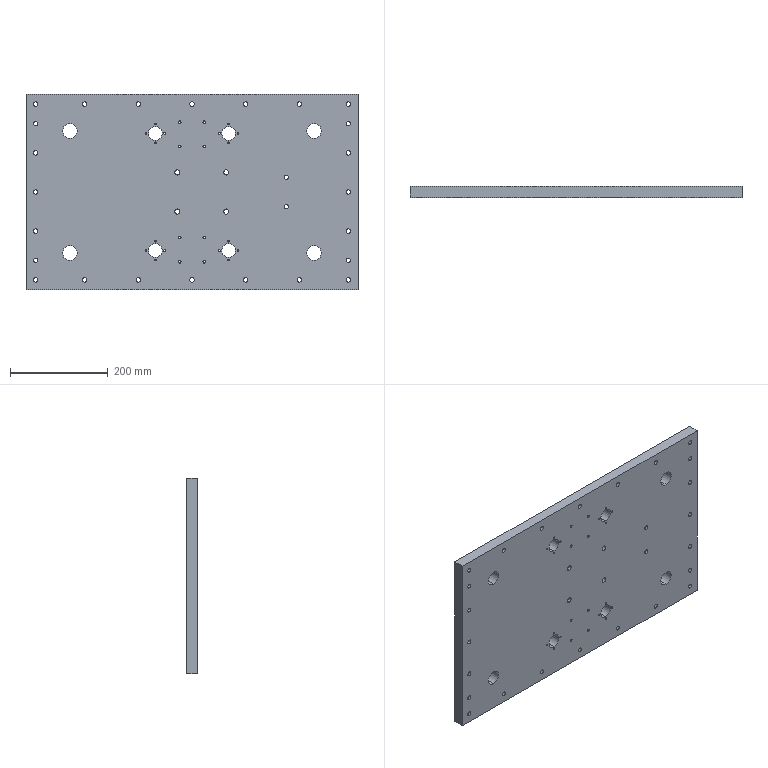Part | STEP file | 1 solid | 266 faces | box 680 x 22 x 400 mm | volume 5788922 mm3 | cylinder 204 | cone 32 | plane 30 | commonest cylinder face diameters 9 x52 5 x48 15 x48 3.3 x32 10.5 x8 28 x8